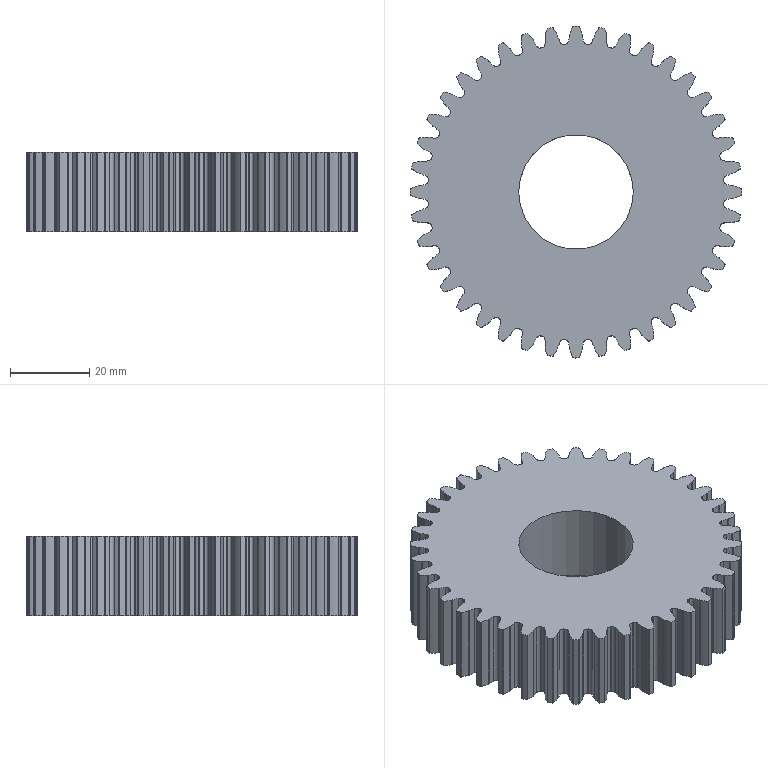Part | NX | features 5003_004_GEAHBB2.0-40-20-A-29 2 | 1 solid | 483 faces | box 84 x 84 x 20 mm | volume 86323 mm3 | cylinder 481 | plane 2 | commonest cylinder face diameters 0.4 x80 2 x80 3.298 x80 26.667 x80 32 x80 75 x40